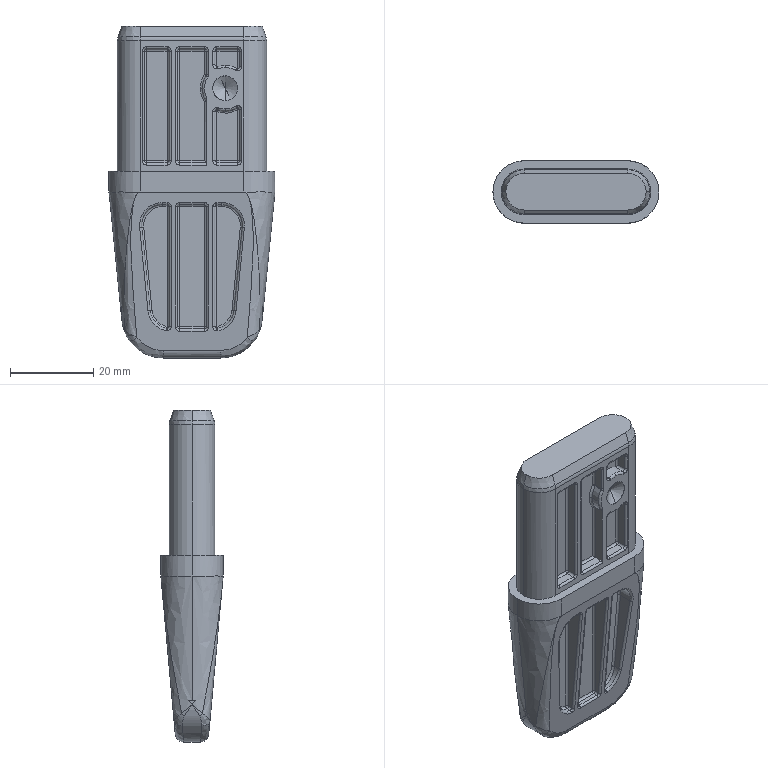Part | STEP file | 101000007784 | 1 solid | 439 faces | box 40 x 15 x 80 mm | volume 24612 mm3 | cylinder 186 | plane 77 | torus 66 | sphere 56 | spline 46 | cone 8 | commonest cylinder face diameters 1 x150 11 x12 10 x8 6 x6 15 x4 20 x4